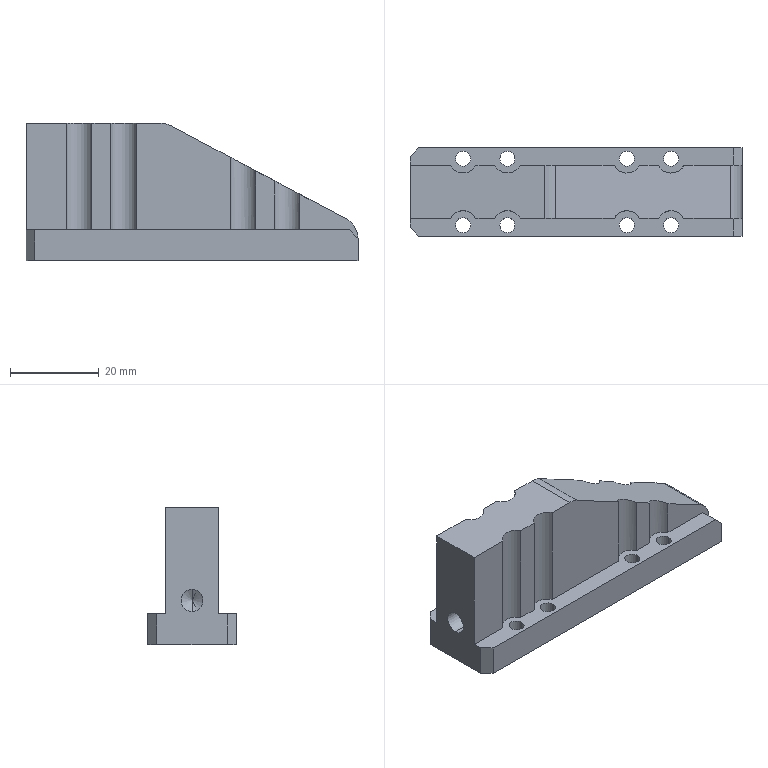Part | STEP file | PN_0032 | 1 solid | 53 faces | box 75 x 20 x 31 mm | volume 24213 mm3 | cylinder 28 | plane 23 | cone 2 | commonest cylinder face diameters 3.4 x16 6.5 x8 5 x2 10 x2